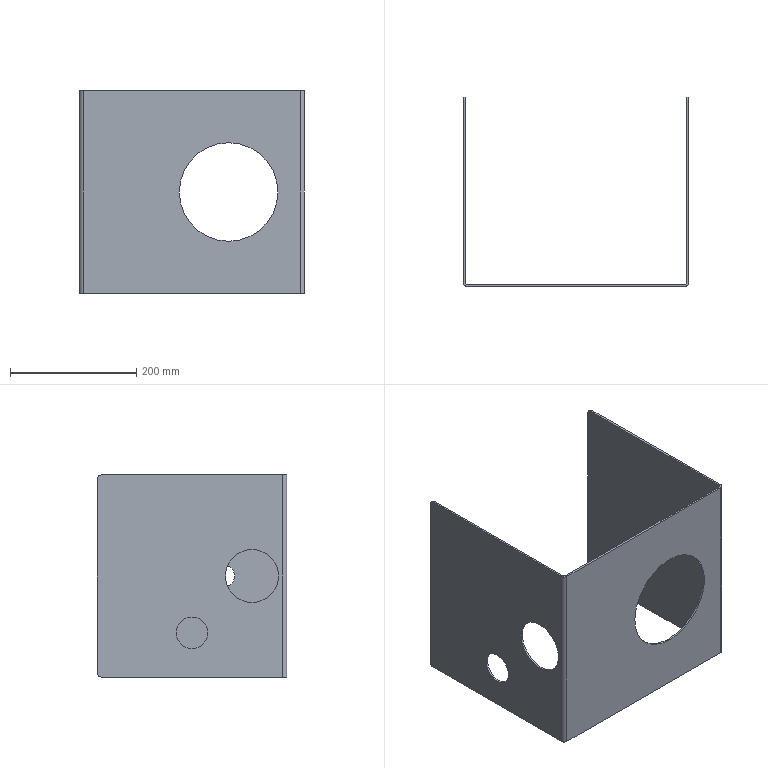Part | SolidWorks | features ICE 4, FlatPattern 1, SMBaseFlange 1, SheetMetal 1 | 1 solid | 34 faces | box 356 x 300 x 320 mm | volume 825456 mm3 | plane 18 | cylinder 16 | commonest cylinder face diameters 12 x6 6 x2 35 x2 50 x2 84 x2 156 x2
STEP:
#1=CARTESIAN_POINT('',(236.,3.,82.));
#2=VERTEX_POINT('',#1);
#3=CARTESIAN_POINT('',(236.,3.,238.));
#4=VERTEX_POINT('',#3);
#5=CARTESIAN_POINT('',(236.,3.,160.));
#6=DIRECTION('',(0.,1.,0.));
#7=DIRECTION('',(0.,0.,1.));
#8=AXIS2_PLACEMENT_3D('',#5,#6,#7);
#9=CIRCLE('',#8,78.);
#10=EDGE_CURVE('',#2,#4,#9,.T.);
#11=ORIENTED_EDGE('',*,*,#10,.T.);
#12=CARTESIAN_POINT('',(236.,0.,238.));
#13=VERTEX_POINT('',#12);
#14=CARTESIAN_POINT('',(236.,10.,238.));
#15=DIRECTION('',(0.,-1.,0.));
#16=VECTOR('',#15,1000.);
#17=LINE('',#14,#16);
#18=EDGE_CURVE('',#4,#13,#17,.T.);
#19=ORIENTED_EDGE('',*,*,#18,.T.);
#20=CARTESIAN_POINT('',(236.,0.,82.));
#21=VERTEX_POINT('',#20);
#22=CARTESIAN_POINT('',(236.,0.,160.));
#23=DIRECTION('',(0.,-1.,0.));
#24=DIRECTION('',(0.,0.,-1.));
#25=AXIS2_PLACEMENT_3D('',#22,#23,#24);
#26=CIRCLE('',#25,78.);
#27=EDGE_CURVE('',#13,#21,#26,.T.);
#28=ORIENTED_EDGE('',*,*,#27,.T.);
#29=CARTESIAN_POINT('',(236.,10.,82.));
#30=DIRECTION('',(0.,-1.,0.));
#31=VECTOR('',#30,1000.);
#32=LINE('',#29,#31);
#33=EDGE_CURVE('',#2,#21,#32,.T.);
#34=ORIENTED_EDGE('',*,*,#33,.F.);
#35=EDGE_LOOP('',(#11,#19,#28,#34));
#36=FACE_OUTER_BOUND('',#35,.T.);
#37=CARTESIAN_POINT('',(236.,10.,160.));
#38=DIRECTION('',(0.,-1.,0.));
#39=DIRECTION('',(0.,0.,-1.));
#40=AXIS2_PLACEMENT_3D('',#37,#38,#39);
#41=CYLINDRICAL_SURFACE('',#40,78.);
#42=ADVANCED_FACE('',(#36),#41,.F.);
#43=CARTESIAN_POINT('',(356.,100.,142.5));
#44=VERTEX_POINT('',#43);
#45=CARTESIAN_POINT('',(356.,100.,177.5));
#46=VERTEX_POINT('',#45);
#47=CARTESIAN_POINT('',(356.,100.,160.));
#48=DIRECTION('',(-1.,0.,0.));
#49=DIRECTION('',(0.,0.,1.));
#50=AXIS2_PLACEMENT_3D('',#47,#48,#49);
#51=CIRCLE('',#50,17.5);
#52=EDGE_CURVE('',#44,#46,#51,.T.);
#53=ORIENTED_EDGE('',*,*,#52,.F.);
#54=CARTESIAN_POINT('',(353.,100.,142.5));
#55=VERTEX_POINT('',#54);
#56=CARTESIAN_POINT('',(363.,100.,142.5));
#57=DIRECTION('',(-1.,0.,0.));
#58=VECTOR('',#57,1000.);
#59=LINE('',#56,#58);
#60=EDGE_CURVE('',#44,#55,#59,.T.);
#61=ORIENTED_EDGE('',*,*,#60,.T.);
#62=CARTESIAN_POINT('',(353.,100.,177.5));
#63=VERTEX_POINT('',#62);
#64=CARTESIAN_POINT('',(353.,100.,160.));
#65=DIRECTION('',(-1.,0.,0.));
#66=DIRECTION('',(0.,0.,1.));
#67=AXIS2_PLACEMENT_3D('',#64,#65,#66);
#68=CIRCLE('',#67,17.5);
#69=EDGE_CURVE('',#55,#63,#68,.T.);
#70=ORIENTED_EDGE('',*,*,#69,.T.);
#71=CARTESIAN_POINT('',(363.,100.,177.5));
#72=DIRECTION('',(-1.,0.,0.));
#73=VECTOR('',#72,1000.);
#74=LINE('',#71,#73);
#75=EDGE_CURVE('',#46,#63,#74,.T.);
#76=ORIENTED_EDGE('',*,*,#75,.F.);
#77=EDGE_LOOP('',(#53,#61,#70,#76));
#78=FACE_OUTER_BOUND('',#77,.T.);
#79=CARTESIAN_POINT('',(363.,100.,160.));
#80=DIRECTION('',(-1.,0.,0.));
#81=DIRECTION('',(0.,0.,1.));
#82=AXIS2_PLACEMENT_3D('',#79,#80,#81);
#83=CYLINDRICAL_SURFACE('',#82,17.5);
#84=ADVANCED_FACE('',(#78),#83,.F.);
#85=CARTESIAN_POINT('',(3.,55.,202.));
#86=VERTEX_POINT('',#85);
#87=CARTESIAN_POINT('',(3.,55.,118.));
#88=VERTEX_POINT('',#87);
#89=CARTESIAN_POINT('',(3.,55.,160.));
#90=DIRECTION('',(1.,0.,0.));
#91=DIRECTION('',(0.,0.,-1.));
#92=AXIS2_PLACEMENT_3D('',#89,#90,#91);
#93=CIRCLE('',#92,42.);
#94=EDGE_CURVE('',#86,#88,#93,.T.);
#95=ORIENTED_EDGE('',*,*,#94,.T.);
#96=CARTESIAN_POINT('',(0.,55.,118.));
#97=VERTEX_POINT('',#96);
#98=CARTESIAN_POINT('',(10.,55.,118.));
#99=DIRECTION('',(-1.,0.,0.));
#100=VECTOR('',#99,1000.);
#101=LINE('',#98,#100);
#102=EDGE_CURVE('',#88,#97,#101,.T.);
#103=ORIENTED_EDGE('',*,*,#102,.T.);
#104=CARTESIAN_POINT('',(0.,55.,202.));
#105=VERTEX_POINT('',#104);
#106=CARTESIAN_POINT('',(0.,55.,160.));
#107=DIRECTION('',(-1.,0.,0.));
#108=DIRECTION('',(0.,0.,1.));
#109=AXIS2_PLACEMENT_3D('',#106,#107,#108);
#110=CIRCLE('',#109,42.);
#111=EDGE_CURVE('',#97,#105,#110,.T.);
#112=ORIENTED_EDGE('',*,*,#111,.T.);
#113=CARTESIAN_POINT('',(10.,55.,202.));
#114=DIRECTION('',(-1.,0.,0.));
#115=VECTOR('',#114,1000.);
#116=LINE('',#113,#115);
#117=EDGE_CURVE('',#86,#105,#116,.T.);
#118=ORIENTED_EDGE('',*,*,#117,.F.);
#119=EDGE_LOOP('',(#95,#103,#112,#118));
#120=FACE_OUTER_BOUND('',#119,.T.);
#121=CARTESIAN_POINT('',(10.,55.,160.));
#122=DIRECTION('',(-1.,0.,0.));
#123=DIRECTION('',(0.,0.,1.));
#124=AXIS2_PLACEMENT_3D('',#121,#122,#123);
#125=CYLINDRICAL_SURFACE('',#124,42.);
#126=ADVANCED_FACE('',(#120),#125,.F.);
#127=CARTESIAN_POINT('',(3.,150.,95.));
#128=VERTEX_POINT('',#127);
#129=CARTESIAN_POINT('',(3.,150.,45.));
#130=VERTEX_POINT('',#129);
#131=CARTESIAN_POINT('',(3.,150.,70.));
#132=DIRECTION('',(1.,0.,0.));
#133=DIRECTION('',(0.,0.,-1.));
#134=AXIS2_PLACEMENT_3D('',#131,#132,#133);
#135=CIRCLE('',#134,25.);
#136=EDGE_CURVE('',#128,#130,#135,.T.);
#137=ORIENTED_EDGE('',*,*,#136,.T.);
#138=CARTESIAN_POINT('',(0.,150.,45.));
#139=VERTEX_POINT('',#138);
#140=CARTESIAN_POINT('',(10.,150.,45.));
#141=DIRECTION('',(-1.,0.,0.));
#142=VECTOR('',#141,1000.);
#143=LINE('',#140,#142);
#144=EDGE_CURVE('',#130,#139,#143,.T.);
#145=ORIENTED_EDGE('',*,*,#144,.T.);
#146=CARTESIAN_POINT('',(0.,150.,95.));
#147=VERTEX_POINT('',#146);
#148=CARTESIAN_POINT('',(0.,150.,70.));
#149=DIRECTION('',(-1.,0.,0.));
#150=DIRECTION('',(0.,0.,1.));
#151=AXIS2_PLACEMENT_3D('',#148,#149,#150);
#152=CIRCLE('',#151,25.);
#153=EDGE_CURVE('',#139,#147,#152,.T.);
#154=ORIENTED_EDGE('',*,*,#153,.T.);
#155=CARTESIAN_POINT('',(10.,150.,95.));
#156=DIRECTION('',(-1.,0.,0.));
#157=VECTOR('',#156,1000.);
#158=LINE('',#155,#157);
#159=EDGE_CURVE('',#128,#147,#158,.T.);
#160=ORIENTED_EDGE('',*,*,#159,.F.);
#161=EDGE_LOOP('',(#137,#145,#154,#160));
#162=FACE_OUTER_BOUND('',#161,.T.);
#163=CARTESIAN_POINT('',(10.,150.,70.));
#164=DIRECTION('',(-1.,0.,0.));
#165=DIRECTION('',(0.,0.,1.));
#166=AXIS2_PLACEMENT_3D('',#163,#164,#165);
#167=CYLINDRICAL_SURFACE('',#166,25.);
#168=ADVANCED_FACE('',(#162),#167,.F.);
#169=CARTESIAN_POINT('',(356.,100.,160.));
#170=DIRECTION('',(-1.,0.,0.));
#171=DIRECTION('',(0.,0.,1.));
#172=AXIS2_PLACEMENT_3D('',#169,#170,#171);
#173=CIRCLE('',#172,17.5);
#174=EDGE_CURVE('',#46,#44,#173,.T.);
#175=ORIENTED_EDGE('',*,*,#174,.T.);
#176=ORIENTED_EDGE('',*,*,#52,.T.);
#177=EDGE_LOOP('',(#175,#176));
#178=FACE_BOUND('',#177,.T.);
#179=CARTESIAN_POINT('',(356.,294.,0.));
#180=VERTEX_POINT('',#179);
#181=CARTESIAN_POINT('',(356.,300.,6.));
#182=VERTEX_POINT('',#181);
#183=CARTESIAN_POINT('',(356.,294.,6.));
#184=DIRECTION('',(1.,0.,0.));
#185=DIRECTION('',(0.,0.,1.));
#186=AXIS2_PLACEMENT_3D('',#183,#184,#185);
#187=CIRCLE('',#186,6.);
#188=EDGE_CURVE('',#180,#182,#187,.T.);
#189=ORIENTED_EDGE('',*,*,#188,.T.);
#190=CARTESIAN_POINT('',(356.,300.,314.));
#191=VERTEX_POINT('',#190);
#192=CARTESIAN_POINT('',(356.,300.,320.));
#193=DIRECTION('',(0.,0.,-1.));
#194=VECTOR('',#193,1000.);
#195=LINE('',#192,#194);
#196=EDGE_CURVE('',#191,#182,#195,.T.);
#197=ORIENTED_EDGE('',*,*,#196,.F.);
#198=CARTESIAN_POINT('',(356.,294.,320.));
#199=VERTEX_POINT('',#198);
#200=CARTESIAN_POINT('',(356.,294.,314.));
#201=DIRECTION('',(1.,0.,0.));
#202=DIRECTION('',(0.,0.,1.));
#203=AXIS2_PLACEMENT_3D('',#200,#201,#202);
#204=CIRCLE('',#203,6.);
#205=EDGE_CURVE('',#191,#199,#204,.T.);
#206=ORIENTED_EDGE('',*,*,#205,.T.);
#207=CARTESIAN_POINT('',(356.,6.,320.));
#208=VERTEX_POINT('',#207);
#209=CARTESIAN_POINT('',(356.,0.,320.));
#210=DIRECTION('',(0.,1.,0.));
#211=VECTOR('',#210,1000.);
#212=LINE('',#209,#211);
#213=EDGE_CURVE('',#208,#199,#212,.T.);
#214=ORIENTED_EDGE('',*,*,#213,.F.);
#215=CARTESIAN_POINT('',(356.,6.,0.));
#216=VERTEX_POINT('',#215);
#217=CARTESIAN_POINT('',(356.,6.,320.));
#218=DIRECTION('',(0.,0.,-1.));
#219=VECTOR('',#218,1000.);
#220=LINE('',#217,#219);
#221=EDGE_CURVE('',#208,#216,#220,.T.);
#222=ORIENTED_EDGE('',*,*,#221,.T.);
#223=CARTESIAN_POINT('',(356.,0.,0.));
#224=DIRECTION('',(0.,1.,0.));
#225=VECTOR('',#224,1000.);
#226=LINE('',#223,#225);
#227=EDGE_CURVE('',#216,#180,#226,.T.);
#228=ORIENTED_EDGE('',*,*,#227,.T.);
#229=EDGE_LOOP('',(#189,#197,#206,#214,#222,#228));
#230=FACE_OUTER_BOUND('',#229,.T.);
#231=CARTESIAN_POINT('',(356.,0.,320.));
#232=DIRECTION('',(-1.,0.,0.));
#233=DIRECTION('',(0.,0.,1.));
#234=AXIS2_PLACEMENT_3D('',#231,#232,#233);
#235=PLANE('',#234);
#236=ADVANCED_FACE('',(#178,#230),#235,.F.);
#237=CARTESIAN_POINT('',(353.,100.,160.));
#238=DIRECTION('',(-1.,0.,0.));
#239=DIRECTION('',(0.,0.,1.));
#240=AXIS2_PLACEMENT_3D('',#237,#238,#239);
#241=CIRCLE('',#240,17.5);
#242=EDGE_CURVE('',#63,#55,#241,.T.);
#243=ORIENTED_EDGE('',*,*,#242,.F.);
#244=ORIENTED_EDGE('',*,*,#69,.F.);
#245=EDGE_LOOP('',(#243,#244));
#246=FACE_BOUND('',#245,.T.);
#247=CARTESIAN_POINT('',(353.,300.,314.));
#248=VERTEX_POINT('',#247);
#249=CARTESIAN_POINT('',(353.,300.,6.));
#250=VERTEX_POINT('',#249);
#251=CARTESIAN_POINT('',(353.,300.,320.));
#252=DIRECTION('',(0.,0.,-1.));
#253=VECTOR('',#252,1000.);
#254=LINE('',#251,#253);
#255=EDGE_CURVE('',#248,#250,#254,.T.);
#256=ORIENTED_EDGE('',*,*,#255,.T.);
#257=CARTESIAN_POINT('',(353.,294.,0.));
#258=VERTEX_POINT('',#257);
#259=CARTESIAN_POINT('',(353.,294.,6.));
#260=DIRECTION('',(1.,0.,0.));
#261=DIRECTION('',(0.,0.,1.));
#262=AXIS2_PLACEMENT_3D('',#259,#260,#261);
#263=CIRCLE('',#262,6.);
#264=EDGE_CURVE('',#258,#250,#263,.T.);
#265=ORIENTED_EDGE('',*,*,#264,.F.);
#266=CARTESIAN_POINT('',(353.,6.,0.));
#267=VERTEX_POINT('',#266);
#268=CARTESIAN_POINT('',(353.,0.,0.));
#269=DIRECTION('',(0.,1.,0.));
#270=VECTOR('',#269,1000.);
#271=LINE('',#268,#270);
#272=EDGE_CURVE('',#267,#258,#271,.T.);
#273=ORIENTED_EDGE('',*,*,#272,.F.);
#274=CARTESIAN_POINT('',(353.,6.,320.));
#275=VERTEX_POINT('',#274);
#276=CARTESIAN_POINT('',(353.,6.,320.));
#277=DIRECTION('',(0.,0.,-1.));
#278=VECTOR('',#277,1000.);
#279=LINE('',#276,#278);
#280=EDGE_CURVE('',#275,#267,#279,.T.);
#281=ORIENTED_EDGE('',*,*,#280,.F.);
#282=CARTESIAN_POINT('',(353.,294.,320.));
#283=VERTEX_POINT('',#282);
#284=CARTESIAN_POINT('',(353.,0.,320.));
#285=DIRECTION('',(0.,1.,0.));
#286=VECTOR('',#285,1000.);
#287=LINE('',#284,#286);
#288=EDGE_CURVE('',#275,#283,#287,.T.);
#289=ORIENTED_EDGE('',*,*,#288,.T.);
#290=CARTESIAN_POINT('',(353.,294.,314.));
#291=DIRECTION('',(1.,0.,0.));
#292=DIRECTION('',(0.,0.,1.));
#293=AXIS2_PLACEMENT_3D('',#290,#291,#292);
#294=CIRCLE('',#293,6.);
#295=EDGE_CURVE('',#248,#283,#294,.T.);
#296=ORIENTED_EDGE('',*,*,#295,.F.);
#297=EDGE_LOOP('',(#256,#265,#273,#281,#289,#296));
#298=FACE_OUTER_BOUND('',#297,.T.);
#299=CARTESIAN_POINT('',(353.,0.,320.));
#300=DIRECTION('',(-1.,0.,0.));
#301=DIRECTION('',(0.,0.,1.));
#302=AXIS2_PLACEMENT_3D('',#299,#300,#301);
#303=PLANE('',#302);
#304=ADVANCED_FACE('',(#246,#298),#303,.T.);
#305=ORIENTED_EDGE('',*,*,#196,.T.);
#306=CARTESIAN_POINT('',(353.,300.,6.));
#307=DIRECTION('',(1.,0.,0.));
#308=VECTOR('',#307,1000.);
#309=LINE('',#306,#308);
#310=EDGE_CURVE('',#250,#182,#309,.T.);
#311=ORIENTED_EDGE('',*,*,#310,.F.);
#312=ORIENTED_EDGE('',*,*,#255,.F.);
#313=CARTESIAN_POINT('',(353.,300.,314.));
#314=DIRECTION('',(1.,0.,0.));
#315=VECTOR('',#314,1000.);
#316=LINE('',#313,#315);
#317=EDGE_CURVE('',#248,#191,#316,.T.);
#318=ORIENTED_EDGE('',*,*,#317,.T.);
#319=EDGE_LOOP('',(#305,#311,#312,#318));
#320=FACE_OUTER_BOUND('',#319,.T.);
#321=CARTESIAN_POINT('',(353.,300.,320.));
#322=DIRECTION('',(0.,1.,0.));
#323=DIRECTION('',(0.,0.,1.));
#324=AXIS2_PLACEMENT_3D('',#321,#322,#323);
#325=PLANE('',#324);
#326=ADVANCED_FACE('',(#320),#325,.T.);
#327=ORIENTED_EDGE('',*,*,#94,.F.);
#328=CARTESIAN_POINT('',(3.,55.,160.));
#329=DIRECTION('',(1.,0.,0.));
#330=DIRECTION('',(0.,0.,-1.));
#331=AXIS2_PLACEMENT_3D('',#328,#329,#330);
#332=CIRCLE('',#331,42.);
#333=EDGE_CURVE('',#88,#86,#332,.T.);
#334=ORIENTED_EDGE('',*,*,#333,.F.);
#335=EDGE_LOOP('',(#327,#334));
#336=FACE_BOUND('',#335,.T.);
#337=ORIENTED_EDGE('',*,*,#136,.F.);
#338=CARTESIAN_POINT('',(3.,150.,70.));
#339=DIRECTION('',(1.,0.,0.));
#340=DIRECTION('',(0.,0.,-1.));
#341=AXIS2_PLACEMENT_3D('',#338,#339,#340);
#342=CIRCLE('',#341,25.);
#343=EDGE_CURVE('',#130,#128,#342,.T.);
#344=ORIENTED_EDGE('',*,*,#343,.F.);
#345=EDGE_LOOP('',(#337,#344));
#346=FACE_BOUND('',#345,.T.);
#347=CARTESIAN_POINT('',(3.,294.,0.));
#348=VERTEX_POINT('',#347);
#349=CARTESIAN_POINT('',(3.,6.,0.));
#350=VERTEX_POINT('',#349);
#351=CARTESIAN_POINT('',(3.,0.,0.));
#352=DIRECTION('',(0.,-1.,0.));
#353=VECTOR('',#352,1000.);
#354=LINE('',#351,#353);
#355=EDGE_CURVE('',#348,#350,#354,.T.);
#356=ORIENTED_EDGE('',*,*,#355,.F.);
#357=CARTESIAN_POINT('',(3.,300.,6.));
#358=VERTEX_POINT('',#357);
#359=CARTESIAN_POINT('',(3.,294.,6.));
#360=DIRECTION('',(-1.,0.,0.));
#361=DIRECTION('',(0.,0.,-1.));
#362=AXIS2_PLACEMENT_3D('',#359,#360,#361);
#363=CIRCLE('',#362,6.);
#364=EDGE_CURVE('',#358,#348,#363,.T.);
#365=ORIENTED_EDGE('',*,*,#364,.F.);
#366=CARTESIAN_POINT('',(3.,300.,314.));
#367=VERTEX_POINT('',#366);
#368=CARTESIAN_POINT('',(3.,300.,320.));
#369=DIRECTION('',(0.,0.,-1.));
#370=VECTOR('',#369,1000.);
#371=LINE('',#368,#370);
#372=EDGE_CURVE('',#367,#358,#371,.T.);
#373=ORIENTED_EDGE('',*,*,#372,.F.);
#374=CARTESIAN_POINT('',(3.,294.,320.));
#375=VERTEX_POINT('',#374);
#376=CARTESIAN_POINT('',(3.,294.,314.));
#377=DIRECTION('',(-1.,0.,0.));
#378=DIRECTION('',(0.,0.,-1.));
#379=AXIS2_PLACEMENT_3D('',#376,#377,#378);
#380=CIRCLE('',#379,6.);
#381=EDGE_CURVE('',#375,#367,#380,.T.);
#382=ORIENTED_EDGE('',*,*,#381,.F.);
#383=CARTESIAN_POINT('',(3.,6.,320.));
#384=VERTEX_POINT('',#383);
#385=CARTESIAN_POINT('',(3.,0.,320.));
#386=DIRECTION('',(0.,-1.,0.));
#387=VECTOR('',#386,1000.);
#388=LINE('',#385,#387);
#389=EDGE_CURVE('',#375,#384,#388,.T.);
#390=ORIENTED_EDGE('',*,*,#389,.T.);
#391=CARTESIAN_POINT('',(3.,6.,320.));
#392=DIRECTION('',(0.,0.,-1.));
#393=VECTOR('',#392,1000.);
#394=LINE('',#391,#393);
#395=EDGE_CURVE('',#384,#350,#394,.T.);
#396=ORIENTED_EDGE('',*,*,#395,.T.);
#397=EDGE_LOOP('',(#356,#365,#373,#382,#390,#396));
#398=FACE_OUTER_BOUND('',#397,.T.);
#399=CARTESIAN_POINT('',(3.,0.,320.));
#400=DIRECTION('',(1.,0.,0.));
#401=DIRECTION('',(0.,0.,-1.));
#402=AXIS2_PLACEMENT_3D('',#399,#400,#401);
#403=PLANE('',#402);
#404=ADVANCED_FACE('',(#336,#346,#398),#403,.T.);
#405=CARTESIAN_POINT('',(0.,55.,160.));
#406=DIRECTION('',(-1.,0.,0.));
#407=DIRECTION('',(0.,0.,1.));
#408=AXIS2_PLACEMENT_3D('',#405,#406,#407);
#409=CIRCLE('',#408,42.);
#410=EDGE_CURVE('',#105,#97,#409,.T.);
#411=ORIENTED_EDGE('',*,*,#410,.F.);
#412=ORIENTED_EDGE('',*,*,#111,.F.);
#413=EDGE_LOOP('',(#411,#412));
#414=FACE_BOUND('',#413,.T.);
#415=CARTESIAN_POINT('',(0.,150.,70.));
#416=DIRECTION('',(-1.,0.,0.));
#417=DIRECTION('',(0.,0.,1.));
#418=AXIS2_PLACEMENT_3D('',#415,#416,#417);
#419=CIRCLE('',#418,25.);
#420=EDGE_CURVE('',#147,#139,#419,.T.);
#421=ORIENTED_EDGE('',*,*,#420,.F.);
#422=ORIENTED_EDGE('',*,*,#153,.F.);
#423=EDGE_LOOP('',(#421,#422));
#424=FACE_BOUND('',#423,.T.);
#425=CARTESIAN_POINT('',(0.,300.,6.));
#426=VERTEX_POINT('',#425);
#427=CARTESIAN_POINT('',(0.,294.,0.));
#428=VERTEX_POINT('',#427);
#429=CARTESIAN_POINT('',(0.,294.,6.));
#430=DIRECTION('',(-1.,0.,0.));
#431=DIRECTION('',(0.,0.,-1.));
#432=AXIS2_PLACEMENT_3D('',#429,#430,#431);
#433=CIRCLE('',#432,6.);
#434=EDGE_CURVE('',#426,#428,#433,.T.);
#435=ORIENTED_EDGE('',*,*,#434,.T.);
#436=CARTESIAN_POINT('',(0.,6.,0.));
#437=VERTEX_POINT('',#436);
#438=CARTESIAN_POINT('',(0.,0.,0.));
#439=DIRECTION('',(0.,-1.,0.));
#440=VECTOR('',#439,1000.);
#441=LINE('',#438,#440);
#442=EDGE_CURVE('',#428,#437,#441,.T.);
#443=ORIENTED_EDGE('',*,*,#442,.T.);
#444=CARTESIAN_POINT('',(0.,6.,320.));
#445=VERTEX_POINT('',#444);
#446=CARTESIAN_POINT('',(0.,6.,320.));
#447=DIRECTION('',(0.,0.,-1.));
#448=VECTOR('',#447,1000.);
#449=LINE('',#446,#448);
#450=EDGE_CURVE('',#445,#437,#449,.T.);
#451=ORIENTED_EDGE('',*,*,#450,.F.);
#452=CARTESIAN_POINT('',(0.,294.,320.));
#453=VERTEX_POINT('',#452);
#454=CARTESIAN_POINT('',(0.,0.,320.));
#455=DIRECTION('',(0.,-1.,0.));
#456=VECTOR('',#455,1000.);
#457=LINE('',#454,#456);
#458=EDGE_CURVE('',#453,#445,#457,.T.);
#459=ORIENTED_EDGE('',*,*,#458,.F.);
#460=CARTESIAN_POINT('',(0.,300.,314.));
#461=VERTEX_POINT('',#460);
#462=CARTESIAN_POINT('',(0.,294.,314.));
#463=DIRECTION('',(-1.,0.,0.));
#464=DIRECTION('',(0.,0.,-1.));
#465=AXIS2_PLACEMENT_3D('',#462,#463,#464);
#466=CIRCLE('',#465,6.);
#467=EDGE_CURVE('',#453,#461,#466,.T.);
#468=ORIENTED_EDGE('',*,*,#467,.T.);
#469=CARTESIAN_POINT('',(0.,300.,320.));
#470=DIRECTION('',(0.,0.,-1.));
#471=VECTOR('',#470,1000.);
#472=LINE('',#469,#471);
#473=EDGE_CURVE('',#461,#426,#472,.T.);
#474=ORIENTED_EDGE('',*,*,#473,.T.);
#475=EDGE_LOOP('',(#435,#443,#451,#459,#468,#474));
#476=FACE_OUTER_BOUND('',#475,.T.);
#477=CARTESIAN_POINT('',(0.,0.,320.));
#478=DIRECTION('',(1.,0.,0.));
#479=DIRECTION('',(0.,0.,-1.));
#480=AXIS2_PLACEMENT_3D('',#477,#478,#479);
#481=PLANE('',#480);
#482=ADVANCED_FACE('',(#414,#424,#476),#481,.F.);
#483=ORIENTED_EDGE('',*,*,#213,.T.);
#484=CARTESIAN_POINT('',(353.,294.,320.));
#485=DIRECTION('',(1.,0.,0.));
#486=VECTOR('',#485,1000.);
#487=LINE('',#484,#486);
#488=EDGE_CURVE('',#283,#199,#487,.T.);
#489=ORIENTED_EDGE('',*,*,#488,.F.);
#490=ORIENTED_EDGE('',*,*,#288,.F.);
#491=CARTESIAN_POINT('',(353.,6.,320.));
#492=DIRECTION('',(1.,0.,0.));
#493=VECTOR('',#492,1000.);
#494=LINE('',#491,#493);
#495=EDGE_CURVE('',#275,#208,#494,.T.);
#496=ORIENTED_EDGE('',*,*,#495,.T.);
#497=EDGE_LOOP('',(#483,#489,#490,#496));
#498=FACE_OUTER_BOUND('',#497,.T.);
#499=CARTESIAN_POINT('',(350.,6.,320.));
#500=DIRECTION('',(0.,0.,1.));
#501=DIRECTION('',(1.,0.,0.));
#502=AXIS2_PLACEMENT_3D('',#499,#500,#501);
#503=PLANE('',#502);
#504=ADVANCED_FACE('',(#498),#503,.T.);
#505=CARTESIAN_POINT('',(3.,300.,6.));
#506=DIRECTION('',(-1.,0.,0.));
#507=VECTOR('',#506,1000.);
#508=LINE('',#505,#507);
#509=EDGE_CURVE('',#358,#426,#508,.T.);
#510=ORIENTED_EDGE('',*,*,#509,.T.);
#511=ORIENTED_EDGE('',*,*,#473,.F.);
#512=CARTESIAN_POINT('',(3.,300.,314.));
#513=DIRECTION('',(-1.,0.,0.));
#514=VECTOR('',#513,1000.);
#515=LINE('',#512,#514);
#516=EDGE_CURVE('',#367,#461,#515,.T.);
#517=ORIENTED_EDGE('',*,*,#516,.F.);
#518=ORIENTED_EDGE('',*,*,#372,.T.);
#519=EDGE_LOOP('',(#510,#511,#517,#518));
#520=FACE_OUTER_BOUND('',#519,.T.);
#521=CARTESIAN_POINT('',(0.,300.,320.));
#522=DIRECTION('',(0.,1.,0.));
#523=DIRECTION('',(0.,0.,1.));
#524=AXIS2_PLACEMENT_3D('',#521,#522,#523);
#525=PLANE('',#524);
#526=ADVANCED_FACE('',(#520),#525,.T.);
#527=CARTESIAN_POINT('',(0.,6.,320.));
#528=DIRECTION('',(1.,0.,0.));
#529=VECTOR('',#528,1000.);
#530=LINE('',#527,#529);
#531=EDGE_CURVE('',#445,#384,#530,.T.);
#532=ORIENTED_EDGE('',*,*,#531,.F.);
#533=CARTESIAN_POINT('',(6.,0.,320.));
#534=VERTEX_POINT('',#533);
#535=CARTESIAN_POINT('',(6.,6.,320.));
#536=DIRECTION('',(0.,0.,1.));
#537=DIRECTION('',(-1.,0.,0.));
#538=AXIS2_PLACEMENT_3D('',#535,#536,#537);
#539=CIRCLE('',#538,6.);
#540=EDGE_CURVE('',#445,#534,#539,.T.);
#541=ORIENTED_EDGE('',*,*,#540,.T.);
#542=CARTESIAN_POINT('',(6.,3.,320.));
#543=VERTEX_POINT('',#542);
#544=CARTESIAN_POINT('',(6.,3.,320.));
#545=DIRECTION('',(0.,-1.,0.));
#546=VECTOR('',#545,1000.);
#547=LINE('',#544,#546);
#548=EDGE_CURVE('',#543,#534,#547,.T.);
#549=ORIENTED_EDGE('',*,*,#548,.F.);
#550=CARTESIAN_POINT('',(6.,6.,320.));
#551=DIRECTION('',(0.,0.,1.));
#552=DIRECTION('',(1.,0.,0.));
#553=AXIS2_PLACEMENT_3D('',#550,#551,#552);
#554=CIRCLE('',#553,3.);
#555=EDGE_CURVE('',#384,#543,#554,.T.);
#556=ORIENTED_EDGE('',*,*,#555,.F.);
#557=EDGE_LOOP('',(#532,#541,#549,#556));
#558=FACE_OUTER_BOUND('',#557,.T.);
#559=CARTESIAN_POINT('',(0.,6.,320.));
#560=DIRECTION('',(0.,0.,1.));
#561=DIRECTION('',(1.,0.,0.));
#562=AXIS2_PLACEMENT_3D('',#559,#560,#561);
#563=PLANE('',#562);
#564=ADVANCED_FACE('',(#558),#563,.T.);
#565=CARTESIAN_POINT('',(3.,294.,320.));
#566=DIRECTION('',(-1.,0.,0.));
#567=VECTOR('',#566,1000.);
#568=LINE('',#565,#567);
#569=EDGE_CURVE('',#375,#453,#568,.T.);
#570=ORIENTED_EDGE('',*,*,#569,.T.);
#571=ORIENTED_EDGE('',*,*,#458,.T.);
#572=ORIENTED_EDGE('',*,*,#531,.T.);
#573=ORIENTED_EDGE('',*,*,#389,.F.);
#574=EDGE_LOOP('',(#570,#571,#572,#573));
#575=FACE_OUTER_BOUND('',#574,.T.);
#576=CARTESIAN_POINT('',(6.,3.,320.));
#577=DIRECTION('',(0.,0.,1.));
#578=DIRECTION('',(1.,0.,0.));
#579=AXIS2_PLACEMENT_3D('',#576,#577,#578);
#580=PLANE('',#579);
#581=ADVANCED_FACE('',(#575),#580,.T.);
#582=CARTESIAN_POINT('',(6.,0.,0.));
#583=VERTEX_POINT('',#582);
#584=CARTESIAN_POINT('',(6.,3.,0.));
#585=VERTEX_POINT('',#584);
#586=CARTESIAN_POINT('',(6.,0.,0.));
#587=DIRECTION('',(0.,1.,0.));
#588=VECTOR('',#587,1000.);
#589=LINE('',#586,#588);
#590=EDGE_CURVE('',#583,#585,#589,.T.);
#591=ORIENTED_EDGE('',*,*,#590,.F.);
#592=CARTESIAN_POINT('',(6.,6.,0.));
#593=DIRECTION('',(0.,0.,1.));
#594=DIRECTION('',(-1.,0.,0.));
#595=AXIS2_PLACEMENT_3D('',#592,#593,#594);
#596=CIRCLE('',#595,6.);
#597=EDGE_CURVE('',#437,#583,#596,.T.);
#598=ORIENTED_EDGE('',*,*,#597,.F.);
#599=CARTESIAN_POINT('',(3.,6.,0.));
#600=DIRECTION('',(-1.,0.,0.));
#601=VECTOR('',#600,1000.);
#602=LINE('',#599,#601);
#603=EDGE_CURVE('',#350,#437,#602,.T.);
#604=ORIENTED_EDGE('',*,*,#603,.F.);
#605=CARTESIAN_POINT('',(6.,6.,0.));
#606=DIRECTION('',(0.,0.,1.));
#607=DIRECTION('',(1.,0.,0.));
#608=AXIS2_PLACEMENT_3D('',#605,#606,#607);
#609=CIRCLE('',#608,3.);
#610=EDGE_CURVE('',#350,#585,#609,.T.);
#611=ORIENTED_EDGE('',*,*,#610,.T.);
#612=EDGE_LOOP('',(#591,#598,#604,#611));
#613=FACE_OUTER_BOUND('',#612,.T.);
#614=CARTESIAN_POINT('',(6.,0.,0.));
#615=DIRECTION('',(0.,0.,-1.));
#616=DIRECTION('',(-1.,0.,0.));
#617=AXIS2_PLACEMENT_3D('',#614,#615,#616);
#618=PLANE('',#617);
#619=ADVANCED_FACE('',(#613),#618,.T.);
#620=CARTESIAN_POINT('',(350.,0.,0.));
#621=VERTEX_POINT('',#620);
#622=CARTESIAN_POINT('',(0.,0.,0.));
#623=DIRECTION('',(1.,0.,0.));
#624=VECTOR('',#623,1000.);
#625=LINE('',#622,#624);
#626=EDGE_CURVE('',#583,#621,#625,.T.);
#627=ORIENTED_EDGE('',*,*,#626,.F.);
#628=ORIENTED_EDGE('',*,*,#590,.T.);
#629=CARTESIAN_POINT('',(350.,3.,0.));
#630=VERTEX_POINT('',#629);
#631=CARTESIAN_POINT('',(0.,3.,0.));
#632=DIRECTION('',(1.,0.,0.));
#633=VECTOR('',#632,1000.);
#634=LINE('',#631,#633);
#635=EDGE_CURVE('',#585,#630,#634,.T.);
#636=ORIENTED_EDGE('',*,*,#635,.T.);
#637=CARTESIAN_POINT('',(350.,3.,0.));
#638=DIRECTION('',(0.,-1.,0.));
#639=VECTOR('',#638,1000.);
#640=LINE('',#637,#639);
#641=EDGE_CURVE('',#630,#621,#640,.T.);
#642=ORIENTED_EDGE('',*,*,#641,.T.);
#643=EDGE_LOOP('',(#627,#628,#636,#642));
#644=FACE_OUTER_BOUND('',#643,.T.);
#645=CARTESIAN_POINT('',(3.,6.,0.));
#646=DIRECTION('',(0.,0.,-1.));
#647=DIRECTION('',(-1.,0.,0.));
#648=AXIS2_PLACEMENT_3D('',#645,#646,#647);
#649=PLANE('',#648);
#650=ADVANCED_FACE('',(#644),#649,.T.);
#651=CARTESIAN_POINT('',(350.,0.,320.));
#652=VERTEX_POINT('',#651);
#653=CARTESIAN_POINT('',(350.,3.,320.));
#654=VERTEX_POINT('',#653);
#655=CARTESIAN_POINT('',(350.,0.,320.));
#656=DIRECTION('',(0.,1.,0.));
#657=VECTOR('',#656,1000.);
#658=LINE('',#655,#657);
#659=EDGE_CURVE('',#652,#654,#658,.T.);
#660=ORIENTED_EDGE('',*,*,#659,.F.);
#661=CARTESIAN_POINT('',(350.,6.,320.));
#662=DIRECTION('',(0.,0.,1.));
#663=DIRECTION('',(-1.,0.,0.));
#664=AXIS2_PLACEMENT_3D('',#661,#662,#663);
#665=CIRCLE('',#664,6.);
#666=EDGE_CURVE('',#652,#208,#665,.T.);
#667=ORIENTED_EDGE('',*,*,#666,.T.);
#668=ORIENTED_EDGE('',*,*,#495,.F.);
#669=CARTESIAN_POINT('',(350.,6.,320.));
#670=DIRECTION('',(0.,0.,1.));
#671=DIRECTION('',(1.,0.,0.));
#672=AXIS2_PLACEMENT_3D('',#669,#670,#671);
#673=CIRCLE('',#672,3.);
#674=EDGE_CURVE('',#654,#275,#673,.T.);
#675=ORIENTED_EDGE('',*,*,#674,.F.);
#676=EDGE_LOOP('',(#660,#667,#668,#675));
#677=FACE_OUTER_BOUND('',#676,.T.);
#678=CARTESIAN_POINT('',(350.,0.,320.));
#679=DIRECTION('',(0.,0.,1.));
#680=DIRECTION('',(1.,0.,0.));
#681=AXIS2_PLACEMENT_3D('',#678,#679,#680);
#682=PLANE('',#681);
#683=ADVANCED_FACE('',(#677),#682,.T.);
#684=CARTESIAN_POINT('',(0.,0.,320.));
#685=DIRECTION('',(1.,0.,0.));
#686=VECTOR('',#685,1000.);
#687=LINE('',#684,#686);
#688=EDGE_CURVE('',#534,#652,#687,.T.);
#689=ORIENTED_EDGE('',*,*,#688,.T.);
#690=ORIENTED_EDGE('',*,*,#659,.T.);
#691=CARTESIAN_POINT('',(0.,3.,320.));
#692=DIRECTION('',(1.,0.,0.));
#693=VECTOR('',#692,1000.);
#694=LINE('',#691,#693);
#695=EDGE_CURVE('',#543,#654,#694,.T.);
#696=ORIENTED_EDGE('',*,*,#695,.F.);
#697=ORIENTED_EDGE('',*,*,#548,.T.);
#698=EDGE_LOOP('',(#689,#690,#696,#697));
#699=FACE_OUTER_BOUND('',#698,.T.);
#700=CARTESIAN_POINT('',(353.,6.,320.));
#701=DIRECTION('',(0.,0.,1.));
#702=DIRECTION('',(1.,0.,0.));
#703=AXIS2_PLACEMENT_3D('',#700,#701,#702);
#704=PLANE('',#703);
#705=ADVANCED_FACE('',(#699),#704,.T.);
#706=CARTESIAN_POINT('',(356.,6.,0.));
#707=DIRECTION('',(-1.,0.,0.));
#708=VECTOR('',#707,1000.);
#709=LINE('',#706,#708);
#710=EDGE_CURVE('',#216,#267,#709,.T.);
#711=ORIENTED_EDGE('',*,*,#710,.F.);
#712=CARTESIAN_POINT('',(350.,6.,0.));
#713=DIRECTION('',(0.,0.,1.));
#714=DIRECTION('',(-1.,0.,0.));
#715=AXIS2_PLACEMENT_3D('',#712,#713,#714);
#716=CIRCLE('',#715,6.);
#717=EDGE_CURVE('',#621,#216,#716,.T.);
#718=ORIENTED_EDGE('',*,*,#717,.F.);
#719=ORIENTED_EDGE('',*,*,#641,.F.);
#720=CARTESIAN_POINT('',(350.,6.,0.));
#721=DIRECTION('',(0.,0.,1.));
#722=DIRECTION('',(1.,0.,0.));
#723=AXIS2_PLACEMENT_3D('',#720,#721,#722);
#724=CIRCLE('',#723,3.);
#725=EDGE_CURVE('',#630,#267,#724,.T.);
#726=ORIENTED_EDGE('',*,*,#725,.T.);
#727=EDGE_LOOP('',(#711,#718,#719,#726));
#728=FACE_OUTER_BOUND('',#727,.T.);
#729=CARTESIAN_POINT('',(356.,6.,0.));
#730=DIRECTION('',(0.,0.,-1.));
#731=DIRECTION('',(-1.,0.,0.));
#732=AXIS2_PLACEMENT_3D('',#729,#730,#731);
#733=PLANE('',#732);
#734=ADVANCED_FACE('',(#728),#733,.T.);
#735=CARTESIAN_POINT('',(353.,294.,0.));
#736=DIRECTION('',(1.,0.,0.));
#737=VECTOR('',#736,1000.);
#738=LINE('',#735,#737);
#739=EDGE_CURVE('',#258,#180,#738,.T.);
#740=ORIENTED_EDGE('',*,*,#739,.T.);
#741=ORIENTED_EDGE('',*,*,#227,.F.);
#742=ORIENTED_EDGE('',*,*,#710,.T.);
#743=ORIENTED_EDGE('',*,*,#272,.T.);
#744=EDGE_LOOP('',(#740,#741,#742,#743));
#745=FACE_OUTER_BOUND('',#744,.T.);
#746=CARTESIAN_POINT('',(350.,3.,0.));
#747=DIRECTION('',(0.,0.,-1.));
#748=DIRECTION('',(-1.,0.,0.));
#749=AXIS2_PLACEMENT_3D('',#746,#747,#748);
#750=PLANE('',#749);
#751=ADVANCED_FACE('',(#745),#750,.T.);
#752=ORIENTED_EDGE('',*,*,#725,.F.);
#753=CARTESIAN_POINT('',(350.,3.,320.));
#754=DIRECTION('',(0.,0.,-1.));
#755=VECTOR('',#754,1000.);
#756=LINE('',#753,#755);
#757=EDGE_CURVE('',#654,#630,#756,.T.);
#758=ORIENTED_EDGE('',*,*,#757,.F.);
#759=ORIENTED_EDGE('',*,*,#674,.T.);
#760=ORIENTED_EDGE('',*,*,#280,.T.);
#761=EDGE_LOOP('',(#752,#758,#759,#760));
#762=FACE_OUTER_BOUND('',#761,.T.);
#763=CARTESIAN_POINT('',(350.,6.,320.));
#764=DIRECTION('',(0.,0.,-1.));
#765=DIRECTION('',(-1.,0.,0.));
#766=AXIS2_PLACEMENT_3D('',#763,#764,#765);
#767=CYLINDRICAL_SURFACE('',#766,3.);
#768=ADVANCED_FACE('',(#762),#767,.F.);
#769=ORIENTED_EDGE('',*,*,#10,.F.);
#770=CARTESIAN_POINT('',(236.,3.,160.));
#771=DIRECTION('',(0.,1.,0.));
#772=DIRECTION('',(0.,0.,1.));
#773=AXIS2_PLACEMENT_3D('',#770,#771,#772);
#774=CIRCLE('',#773,78.);
#775=EDGE_CURVE('',#4,#2,#774,.T.);
#776=ORIENTED_EDGE('',*,*,#775,.F.);
#777=EDGE_LOOP('',(#769,#776));
#778=FACE_BOUND('',#777,.T.);
#779=ORIENTED_EDGE('',*,*,#635,.F.);
#780=CARTESIAN_POINT('',(6.,3.,320.));
#781=DIRECTION('',(0.,0.,-1.));
#782=VECTOR('',#781,1000.);
#783=LINE('',#780,#782);
#784=EDGE_CURVE('',#543,#585,#783,.T.);
#785=ORIENTED_EDGE('',*,*,#784,.F.);
#786=ORIENTED_EDGE('',*,*,#695,.T.);
#787=ORIENTED_EDGE('',*,*,#757,.T.);
#788=EDGE_LOOP('',(#779,#785,#786,#787));
#789=FACE_OUTER_BOUND('',#788,.T.);
#790=CARTESIAN_POINT('',(0.,3.,320.));
#791=DIRECTION('',(0.,1.,0.));
#792=DIRECTION('',(0.,0.,1.));
#793=AXIS2_PLACEMENT_3D('',#790,#791,#792);
#794=PLANE('',#793);
#795=ADVANCED_FACE('',(#778,#789),#794,.T.);
#796=ORIENTED_EDGE('',*,*,#610,.F.);
#797=ORIENTED_EDGE('',*,*,#395,.F.);
#798=ORIENTED_EDGE('',*,*,#555,.T.);
#799=ORIENTED_EDGE('',*,*,#784,.T.);
#800=EDGE_LOOP('',(#796,#797,#798,#799));
#801=FACE_OUTER_BOUND('',#800,.T.);
#802=CARTESIAN_POINT('',(6.,6.,320.));
#803=DIRECTION('',(0.,0.,-1.));
#804=DIRECTION('',(-1.,0.,0.));
#805=AXIS2_PLACEMENT_3D('',#802,#803,#804);
#806=CYLINDRICAL_SURFACE('',#805,3.);
#807=ADVANCED_FACE('',(#801),#806,.F.);
#808=ORIENTED_EDGE('',*,*,#597,.T.);
#809=CARTESIAN_POINT('',(6.,0.,320.));
#810=DIRECTION('',(0.,0.,-1.));
#811=VECTOR('',#810,1000.);
#812=LINE('',#809,#811);
#813=EDGE_CURVE('',#534,#583,#812,.T.);
#814=ORIENTED_EDGE('',*,*,#813,.F.);
#815=ORIENTED_EDGE('',*,*,#540,.F.);
#816=ORIENTED_EDGE('',*,*,#450,.T.);
#817=EDGE_LOOP('',(#808,#814,#815,#816));
#818=FACE_OUTER_BOUND('',#817,.T.);
#819=CARTESIAN_POINT('',(6.,6.,320.));
#820=DIRECTION('',(0.,0.,-1.));
#821=DIRECTION('',(-1.,0.,0.));
#822=AXIS2_PLACEMENT_3D('',#819,#820,#821);
#823=CYLINDRICAL_SURFACE('',#822,6.);
#824=ADVANCED_FACE('',(#818),#823,.T.);
#825=CARTESIAN_POINT('',(236.,0.,160.));
#826=DIRECTION('',(0.,-1.,0.));
#827=DIRECTION('',(0.,0.,-1.));
#828=AXIS2_PLACEMENT_3D('',#825,#826,#827);
#829=CIRCLE('',#828,78.);
#830=EDGE_CURVE('',#21,#13,#829,.T.);
#831=ORIENTED_EDGE('',*,*,#830,.F.);
#832=ORIENTED_EDGE('',*,*,#27,.F.);
#833=EDGE_LOOP('',(#831,#832));
#834=FACE_BOUND('',#833,.T.);
#835=ORIENTED_EDGE('',*,*,#626,.T.);
#836=CARTESIAN_POINT('',(350.,0.,320.));
#837=DIRECTION('',(0.,0.,-1.));
#838=VECTOR('',#837,1000.);
#839=LINE('',#836,#838);
#840=EDGE_CURVE('',#652,#621,#839,.T.);
#841=ORIENTED_EDGE('',*,*,#840,.F.);
#842=ORIENTED_EDGE('',*,*,#688,.F.);
#843=ORIENTED_EDGE('',*,*,#813,.T.);
#844=EDGE_LOOP('',(#835,#841,#842,#843));
#845=FACE_OUTER_BOUND('',#844,.T.);
#846=CARTESIAN_POINT('',(0.,0.,320.));
#847=DIRECTION('',(0.,1.,0.));
#848=DIRECTION('',(0.,0.,1.));
#849=AXIS2_PLACEMENT_3D('',#846,#847,#848);
#850=PLANE('',#849);
#851=ADVANCED_FACE('',(#834,#845),#850,.F.);
#852=ORIENTED_EDGE('',*,*,#717,.T.);
#853=ORIENTED_EDGE('',*,*,#221,.F.);
#854=ORIENTED_EDGE('',*,*,#666,.F.);
#855=ORIENTED_EDGE('',*,*,#840,.T.);
#856=EDGE_LOOP('',(#852,#853,#854,#855));
#857=FACE_OUTER_BOUND('',#856,.T.);
#858=CARTESIAN_POINT('',(350.,6.,320.));
#859=DIRECTION('',(0.,0.,-1.));
#860=DIRECTION('',(-1.,0.,0.));
#861=AXIS2_PLACEMENT_3D('',#858,#859,#860);
#862=CYLINDRICAL_SURFACE('',#861,6.);
#863=ADVANCED_FACE('',(#857),#862,.T.);
#864=ORIENTED_EDGE('',*,*,#442,.F.);
#865=CARTESIAN_POINT('',(3.,294.,0.));
#866=DIRECTION('',(-1.,0.,0.));
#867=VECTOR('',#866,1000.);
#868=LINE('',#865,#867);
#869=EDGE_CURVE('',#348,#428,#868,.T.);
#870=ORIENTED_EDGE('',*,*,#869,.F.);
#871=ORIENTED_EDGE('',*,*,#355,.T.);
#872=ORIENTED_EDGE('',*,*,#603,.T.);
#873=EDGE_LOOP('',(#864,#870,#871,#872));
#874=FACE_OUTER_BOUND('',#873,.T.);
#875=CARTESIAN_POINT('',(350.,6.,0.));
#876=DIRECTION('',(0.,0.,1.));
#877=DIRECTION('',(1.,0.,0.));
#878=AXIS2_PLACEMENT_3D('',#875,#876,#877);
#879=PLANE('',#878);
#880=ADVANCED_FACE('',(#874),#879,.F.);
#881=ORIENTED_EDGE('',*,*,#144,.F.);
#882=ORIENTED_EDGE('',*,*,#343,.T.);
#883=ORIENTED_EDGE('',*,*,#159,.T.);
#884=ORIENTED_EDGE('',*,*,#420,.T.);
#885=EDGE_LOOP('',(#881,#882,#883,#884));
#886=FACE_OUTER_BOUND('',#885,.T.);
#887=CARTESIAN_POINT('',(10.,150.,70.));
#888=DIRECTION('',(-1.,0.,0.));
#889=DIRECTION('',(0.,0.,1.));
#890=AXIS2_PLACEMENT_3D('',#887,#888,#889);
#891=CYLINDRICAL_SURFACE('',#890,25.);
#892=ADVANCED_FACE('',(#886),#891,.F.);
#893=ORIENTED_EDGE('',*,*,#102,.F.);
#894=ORIENTED_EDGE('',*,*,#333,.T.);
#895=ORIENTED_EDGE('',*,*,#117,.T.);
#896=ORIENTED_EDGE('',*,*,#410,.T.);
#897=EDGE_LOOP('',(#893,#894,#895,#896));
#898=FACE_OUTER_BOUND('',#897,.T.);
#899=CARTESIAN_POINT('',(10.,55.,160.));
#900=DIRECTION('',(-1.,0.,0.));
#901=DIRECTION('',(0.,0.,1.));
#902=AXIS2_PLACEMENT_3D('',#899,#900,#901);
#903=CYLINDRICAL_SURFACE('',#902,42.);
#904=ADVANCED_FACE('',(#898),#903,.F.);
#905=ORIENTED_EDGE('',*,*,#60,.F.);
#906=ORIENTED_EDGE('',*,*,#174,.F.);
#907=ORIENTED_EDGE('',*,*,#75,.T.);
#908=ORIENTED_EDGE('',*,*,#242,.T.);
#909=EDGE_LOOP('',(#905,#906,#907,#908));
#910=FACE_OUTER_BOUND('',#909,.T.);
#911=CARTESIAN_POINT('',(363.,100.,160.));
#912=DIRECTION('',(-1.,0.,0.));
#913=DIRECTION('',(0.,0.,1.));
#914=AXIS2_PLACEMENT_3D('',#911,#912,#913);
#915=CYLINDRICAL_SURFACE('',#914,17.5);
#916=ADVANCED_FACE('',(#910),#915,.F.);
#917=ORIENTED_EDGE('',*,*,#18,.F.);
#918=ORIENTED_EDGE('',*,*,#775,.T.);
#919=ORIENTED_EDGE('',*,*,#33,.T.);
#920=ORIENTED_EDGE('',*,*,#830,.T.);
#921=EDGE_LOOP('',(#917,#918,#919,#920));
#922=FACE_OUTER_BOUND('',#921,.T.);
#923=CARTESIAN_POINT('',(236.,10.,160.));
#924=DIRECTION('',(0.,-1.,0.));
#925=DIRECTION('',(0.,0.,-1.));
#926=AXIS2_PLACEMENT_3D('',#923,#924,#925);
#927=CYLINDRICAL_SURFACE('',#926,78.);
#928=ADVANCED_FACE('',(#922),#927,.F.);
#929=ORIENTED_EDGE('',*,*,#381,.T.);
#930=ORIENTED_EDGE('',*,*,#516,.T.);
#931=ORIENTED_EDGE('',*,*,#467,.F.);
#932=ORIENTED_EDGE('',*,*,#569,.F.);
#933=EDGE_LOOP('',(#929,#930,#931,#932));
#934=FACE_OUTER_BOUND('',#933,.T.);
#935=CARTESIAN_POINT('',(3.,294.,314.));
#936=DIRECTION('',(1.,0.,0.));
#937=DIRECTION('',(0.,0.,-1.));
#938=AXIS2_PLACEMENT_3D('',#935,#936,#937);
#939=CYLINDRICAL_SURFACE('',#938,6.);
#940=ADVANCED_FACE('',(#934),#939,.T.);
#941=ORIENTED_EDGE('',*,*,#295,.T.);
#942=ORIENTED_EDGE('',*,*,#488,.T.);
#943=ORIENTED_EDGE('',*,*,#205,.F.);
#944=ORIENTED_EDGE('',*,*,#317,.F.);
#945=EDGE_LOOP('',(#941,#942,#943,#944));
#946=FACE_OUTER_BOUND('',#945,.T.);
#947=CARTESIAN_POINT('',(353.,294.,314.));
#948=DIRECTION('',(-1.,0.,0.));
#949=DIRECTION('',(0.,0.,1.));
#950=AXIS2_PLACEMENT_3D('',#947,#948,#949);
#951=CYLINDRICAL_SURFACE('',#950,6.);
#952=ADVANCED_FACE('',(#946),#951,.T.);
#953=ORIENTED_EDGE('',*,*,#364,.T.);
#954=ORIENTED_EDGE('',*,*,#869,.T.);
#955=ORIENTED_EDGE('',*,*,#434,.F.);
#956=ORIENTED_EDGE('',*,*,#509,.F.);
#957=EDGE_LOOP('',(#953,#954,#955,#956));
#958=FACE_OUTER_BOUND('',#957,.T.);
#959=CARTESIAN_POINT('',(3.,294.,6.));
#960=DIRECTION('',(1.,0.,0.));
#961=DIRECTION('',(0.,0.,-1.));
#962=AXIS2_PLACEMENT_3D('',#959,#960,#961);
#963=CYLINDRICAL_SURFACE('',#962,6.);
#964=ADVANCED_FACE('',(#958),#963,.T.);
#965=ORIENTED_EDGE('',*,*,#264,.T.);
#966=ORIENTED_EDGE('',*,*,#310,.T.);
#967=ORIENTED_EDGE('',*,*,#188,.F.);
#968=ORIENTED_EDGE('',*,*,#739,.F.);
#969=EDGE_LOOP('',(#965,#966,#967,#968));
#970=FACE_OUTER_BOUND('',#969,.T.);
#971=CARTESIAN_POINT('',(353.,294.,6.));
#972=DIRECTION('',(-1.,0.,0.));
#973=DIRECTION('',(0.,0.,1.));
#974=AXIS2_PLACEMENT_3D('',#971,#972,#973);
#975=CYLINDRICAL_SURFACE('',#974,6.);
#976=ADVANCED_FACE('',(#970),#975,.T.);
#977=CLOSED_SHELL('',(#42,#84,#126,#168,#236,#304,#326,#404,#482,#504,#526,#564,#581,#619,#650,#683,#705,#734,#751,#768,#795,#807,#824,#851,#863,#880,#892,#904,#916,#928,#940,#952,#964,#976));
#978=MANIFOLD_SOLID_BREP('',#977);
#979=CARTESIAN_POINT('',(0.,0.,0.));
#980=DIRECTION('',(0.,0.,1.));
#981=DIRECTION('',(1.,0.,0.));
#982=AXIS2_PLACEMENT_3D('',#979,#980,#981);
#983=(LENGTH_UNIT()NAMED_UNIT(*)SI_UNIT(.MILLI.,.METRE.));
#984=UNCERTAINTY_MEASURE_WITH_UNIT(LENGTH_MEASURE(0.00001),#983,'','');
#985=(NAMED_UNIT(*)PLANE_ANGLE_UNIT()SI_UNIT($,.RADIAN.));
#986=(NAMED_UNIT(*)SI_UNIT($,.STERADIAN.)SOLID_ANGLE_UNIT());
#987=(GEOMETRIC_REPRESENTATION_CONTEXT(3)GLOBAL_UNCERTAINTY_ASSIGNED_CONTEXT((#984))GLOBAL_UNIT_ASSIGNED_CONTEXT((#983,#985,#986))REPRESENTATION_CONTEXT('',''));
#988=ADVANCED_BREP_SHAPE_REPRESENTATION('',(#978,#982),#987);